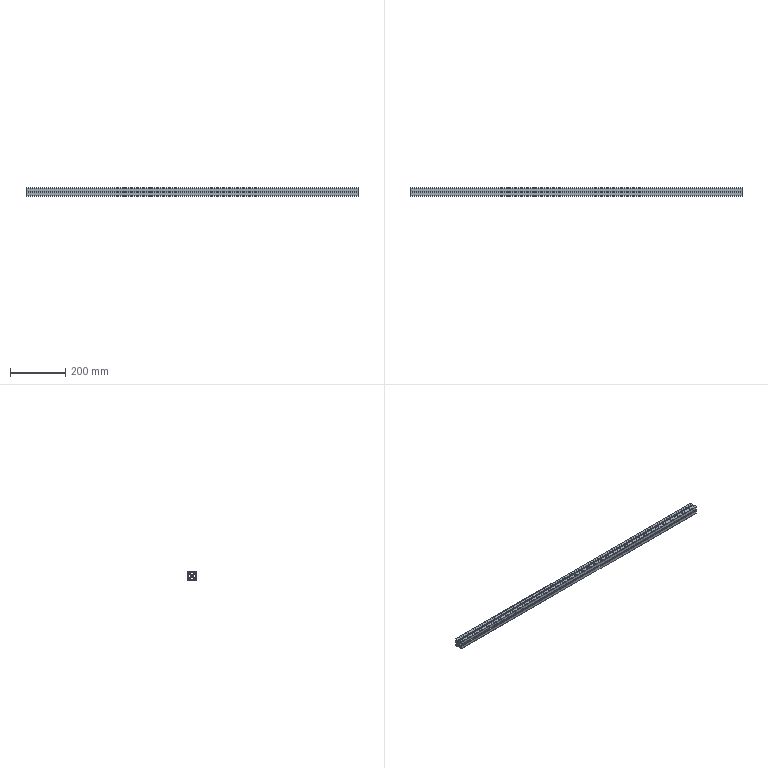Part | SolidWorks | features WeldMemberFeat 1, WeldmentFeature 1 | 1 solid | 64 faces | box 1200 x 30 x 30 mm | volume 478805 mm3 | plane 42 | cylinder 22 | commonest cylinder face diameters 6 x8 15.262 x8 2 x4 5 x2